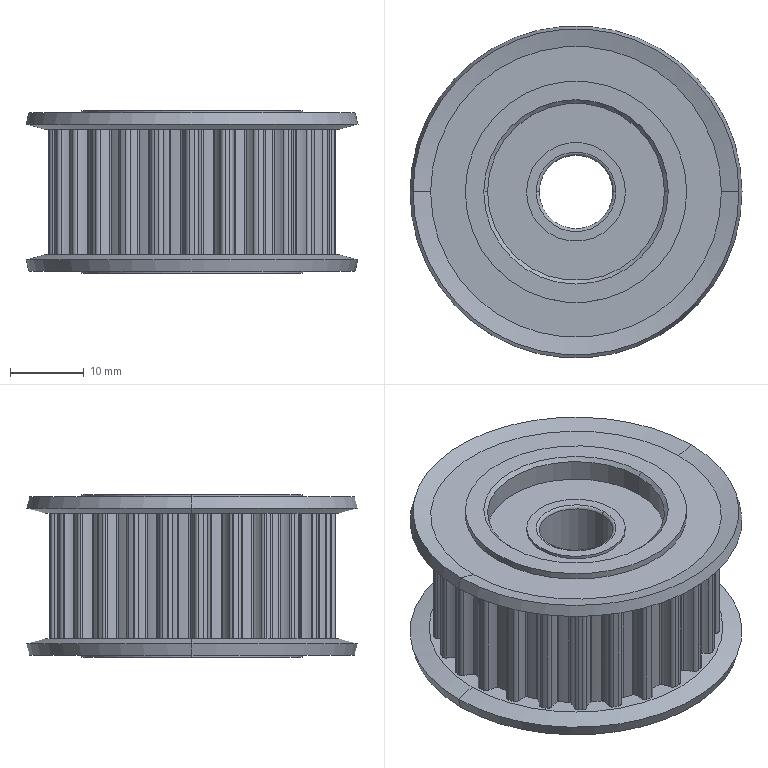Part | SolidWorks | 1 solid | 319 faces | box 45 x 45 x 22 mm | volume 19865 mm3 | cylinder 264 | plane 23 | cone 16 | torus 16 | commonest cylinder face diameters 1.1 x61 0.5 x57 6.55 x53 35.29 x25 38.83 x25 26 x8